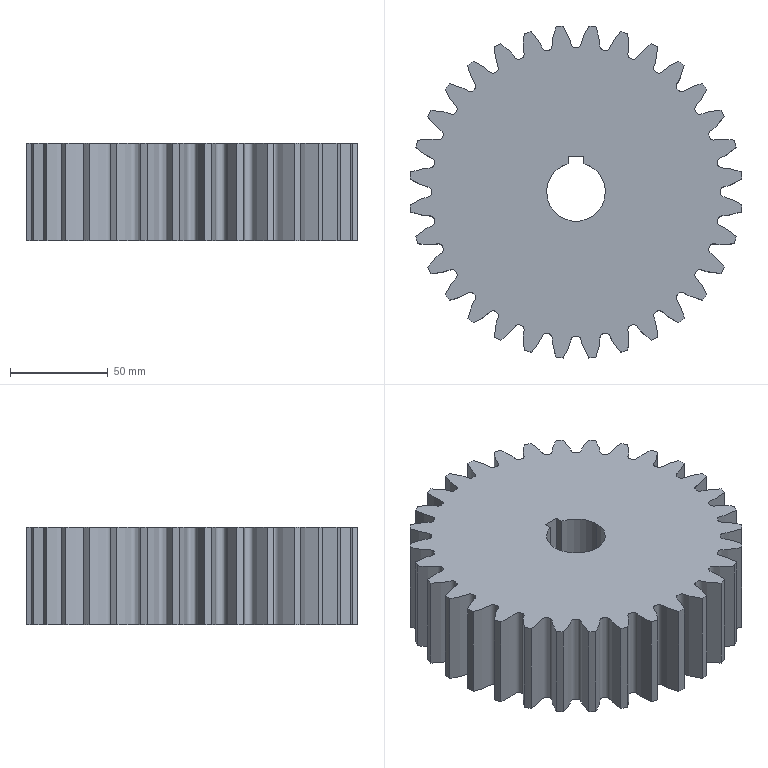Part | STEP file | Spur gear_GearTrax | 1 solid | 72 faces | box 169.505 x 169.505 x 50 mm | volume 949713 mm3 | cylinder 35 | spline 32 | plane 5 | commonest cylinder face diameters 170 x32 30 x3